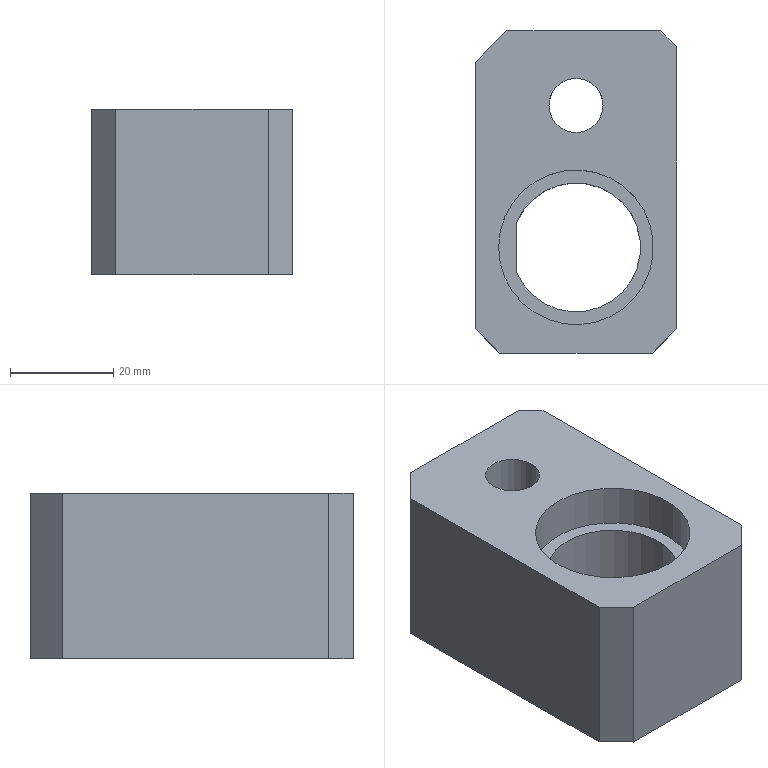Part | STEP file | lll_id3166_x_t | 1 solid | 17 faces | box 39 x 62.5 x 32 mm | volume 54047 mm3 | plane 13 | cylinder 4 | commonest cylinder face diameters 10.5 x1 17 x1 25 x1 30 x1
STEP:
#1=CARTESIAN_POINT('',(481.37,-352.399,60.5));
#2=VERTEX_POINT('',#1);
#3=CARTESIAN_POINT('',(481.37,-342.601,60.5));
#4=VERTEX_POINT('',#3);
#5=CARTESIAN_POINT('',(492.87,-347.5,60.5));
#6=DIRECTION('',(0.,0.,1.));
#7=DIRECTION('',(-1.,0.,0.));
#8=AXIS2_PLACEMENT_3D('',#5,#6,#7);
#9=CIRCLE('',#8,12.5);
#10=EDGE_CURVE('',#2,#4,#9,.T.);
#11=ORIENTED_EDGE('',*,*,#10,.T.);
#12=CARTESIAN_POINT('',(481.37,-316.275,60.5));
#13=DIRECTION('',(0.,-1.,0.));
#14=VECTOR('',#13,1.);
#15=LINE('',#12,#14);
#16=EDGE_CURVE('',#4,#2,#15,.T.);
#17=ORIENTED_EDGE('',*,*,#16,.T.);
#18=EDGE_LOOP('',(#11,#17));
#19=FACE_BOUND('',#18,.T.);
#20=CARTESIAN_POINT('',(507.613,-368.,60.5));
#21=VERTEX_POINT('',#20);
#22=CARTESIAN_POINT('',(478.128,-368.,60.5));
#23=VERTEX_POINT('',#22);
#24=CARTESIAN_POINT('',(492.87,-368.,60.5));
#25=DIRECTION('',(-1.,0.,0.));
#26=VECTOR('',#25,1.);
#27=LINE('',#24,#26);
#28=EDGE_CURVE('',#21,#23,#27,.T.);
#29=ORIENTED_EDGE('',*,*,#28,.T.);
#30=CARTESIAN_POINT('',(473.37,-363.243,60.5));
#31=VERTEX_POINT('',#30);
#32=CARTESIAN_POINT('',(425.566,-315.439,60.5));
#33=DIRECTION('',(0.7071,-0.7071,0.));
#34=VECTOR('',#33,1.);
#35=LINE('',#32,#34);
#36=EDGE_CURVE('',#31,#23,#35,.T.);
#37=ORIENTED_EDGE('',*,*,#36,.F.);
#38=CARTESIAN_POINT('',(473.37,-311.601,60.5));
#39=VERTEX_POINT('',#38);
#40=CARTESIAN_POINT('',(473.37,-347.5,60.5));
#41=DIRECTION('',(0.,1.,0.));
#42=VECTOR('',#41,1.);
#43=LINE('',#40,#42);
#44=EDGE_CURVE('',#31,#39,#43,.T.);
#45=ORIENTED_EDGE('',*,*,#44,.T.);
#46=CARTESIAN_POINT('',(479.471,-305.5,60.5));
#47=VERTEX_POINT('',#46);
#48=CARTESIAN_POINT('',(449.213,-335.758,60.5));
#49=DIRECTION('',(-0.7071,-0.7071,0.));
#50=VECTOR('',#49,1.);
#51=LINE('',#48,#50);
#52=EDGE_CURVE('',#47,#39,#51,.T.);
#53=ORIENTED_EDGE('',*,*,#52,.F.);
#54=CARTESIAN_POINT('',(509.27,-305.5,60.5));
#55=VERTEX_POINT('',#54);
#56=CARTESIAN_POINT('',(492.87,-305.5,60.5));
#57=DIRECTION('',(1.,0.,0.));
#58=VECTOR('',#57,1.);
#59=LINE('',#56,#58);
#60=EDGE_CURVE('',#47,#55,#59,.T.);
#61=ORIENTED_EDGE('',*,*,#60,.T.);
#62=CARTESIAN_POINT('',(512.37,-308.601,60.5));
#63=VERTEX_POINT('',#62);
#64=CARTESIAN_POINT('',(469.887,-266.118,60.5));
#65=DIRECTION('',(-0.7071,0.7071,0.));
#66=VECTOR('',#65,1.);
#67=LINE('',#64,#66);
#68=EDGE_CURVE('',#63,#55,#67,.T.);
#69=ORIENTED_EDGE('',*,*,#68,.F.);
#70=CARTESIAN_POINT('',(512.37,-363.243,60.5));
#71=VERTEX_POINT('',#70);
#72=CARTESIAN_POINT('',(512.37,-347.5,60.5));
#73=DIRECTION('',(0.,-1.,0.));
#74=VECTOR('',#73,1.);
#75=LINE('',#72,#74);
#76=EDGE_CURVE('',#63,#71,#75,.T.);
#77=ORIENTED_EDGE('',*,*,#76,.T.);
#78=CARTESIAN_POINT('',(492.034,-383.579,60.5));
#79=DIRECTION('',(0.7071,0.7071,0.));
#80=VECTOR('',#79,1.);
#81=LINE('',#78,#80);
#82=EDGE_CURVE('',#21,#71,#81,.T.);
#83=ORIENTED_EDGE('',*,*,#82,.F.);
#84=EDGE_LOOP('',(#29,#37,#45,#53,#61,#69,#77,#83));
#85=FACE_BOUND('',#84,.T.);
#86=CARTESIAN_POINT('',(501.37,-320.,60.5));
#87=VERTEX_POINT('',#86);
#88=CARTESIAN_POINT('',(492.87,-320.,60.5));
#89=DIRECTION('',(0.,0.,-1.));
#90=DIRECTION('',(1.,0.,0.));
#91=AXIS2_PLACEMENT_3D('',#88,#89,#90);
#92=CIRCLE('',#91,8.5);
#93=EDGE_CURVE('',#87,#87,#92,.T.);
#94=ORIENTED_EDGE('',*,*,#93,.F.);
#95=EDGE_LOOP('',(#94));
#96=FACE_BOUND('',#95,.T.);
#97=CARTESIAN_POINT('',(424.73,-316.275,60.5));
#98=DIRECTION('',(0.,0.,1.));
#99=DIRECTION('',(-1.,0.,0.));
#100=AXIS2_PLACEMENT_3D('',#97,#98,#99);
#101=PLANE('',#100);
#102=ADVANCED_FACE('',(#19,#85,#96),#101,.F.);
#103=CARTESIAN_POINT('',(477.87,-347.5,92.5));
#104=VERTEX_POINT('',#103);
#105=CARTESIAN_POINT('',(492.87,-347.5,92.5));
#106=DIRECTION('',(0.,0.,1.));
#107=DIRECTION('',(-1.,0.,0.));
#108=AXIS2_PLACEMENT_3D('',#105,#106,#107);
#109=CIRCLE('',#108,15.);
#110=EDGE_CURVE('',#104,#104,#109,.T.);
#111=ORIENTED_EDGE('',*,*,#110,.F.);
#112=EDGE_LOOP('',(#111));
#113=FACE_BOUND('',#112,.T.);
#114=CARTESIAN_POINT('',(498.12,-320.,92.5));
#115=VERTEX_POINT('',#114);
#116=CARTESIAN_POINT('',(492.87,-320.,92.5));
#117=DIRECTION('',(0.,0.,-1.));
#118=DIRECTION('',(1.,0.,0.));
#119=AXIS2_PLACEMENT_3D('',#116,#117,#118);
#120=CIRCLE('',#119,5.25);
#121=EDGE_CURVE('',#115,#115,#120,.T.);
#122=ORIENTED_EDGE('',*,*,#121,.T.);
#123=EDGE_LOOP('',(#122));
#124=FACE_BOUND('',#123,.T.);
#125=CARTESIAN_POINT('',(512.37,-363.243,92.5));
#126=VERTEX_POINT('',#125);
#127=CARTESIAN_POINT('',(512.37,-308.601,92.5));
#128=VERTEX_POINT('',#127);
#129=CARTESIAN_POINT('',(512.37,-347.5,92.5));
#130=DIRECTION('',(0.,1.,0.));
#131=VECTOR('',#130,1.);
#132=LINE('',#129,#131);
#133=EDGE_CURVE('',#126,#128,#132,.T.);
#134=ORIENTED_EDGE('',*,*,#133,.T.);
#135=CARTESIAN_POINT('',(509.27,-305.5,92.5));
#136=VERTEX_POINT('',#135);
#137=CARTESIAN_POINT('',(469.887,-266.118,92.5));
#138=DIRECTION('',(0.7071,-0.7071,0.));
#139=VECTOR('',#138,1.);
#140=LINE('',#137,#139);
#141=EDGE_CURVE('',#136,#128,#140,.T.);
#142=ORIENTED_EDGE('',*,*,#141,.F.);
#143=CARTESIAN_POINT('',(479.471,-305.5,92.5));
#144=VERTEX_POINT('',#143);
#145=CARTESIAN_POINT('',(492.87,-305.5,92.5));
#146=DIRECTION('',(-1.,0.,0.));
#147=VECTOR('',#146,1.);
#148=LINE('',#145,#147);
#149=EDGE_CURVE('',#136,#144,#148,.T.);
#150=ORIENTED_EDGE('',*,*,#149,.T.);
#151=CARTESIAN_POINT('',(473.37,-311.601,92.5));
#152=VERTEX_POINT('',#151);
#153=CARTESIAN_POINT('',(449.213,-335.758,92.5));
#154=DIRECTION('',(0.7071,0.7071,0.));
#155=VECTOR('',#154,1.);
#156=LINE('',#153,#155);
#157=EDGE_CURVE('',#152,#144,#156,.T.);
#158=ORIENTED_EDGE('',*,*,#157,.F.);
#159=CARTESIAN_POINT('',(473.37,-363.243,92.5));
#160=VERTEX_POINT('',#159);
#161=CARTESIAN_POINT('',(473.37,-347.5,92.5));
#162=DIRECTION('',(0.,-1.,0.));
#163=VECTOR('',#162,1.);
#164=LINE('',#161,#163);
#165=EDGE_CURVE('',#152,#160,#164,.T.);
#166=ORIENTED_EDGE('',*,*,#165,.T.);
#167=CARTESIAN_POINT('',(478.128,-368.,92.5));
#168=VERTEX_POINT('',#167);
#169=CARTESIAN_POINT('',(425.566,-315.439,92.5));
#170=DIRECTION('',(-0.7071,0.7071,0.));
#171=VECTOR('',#170,1.);
#172=LINE('',#169,#171);
#173=EDGE_CURVE('',#168,#160,#172,.T.);
#174=ORIENTED_EDGE('',*,*,#173,.F.);
#175=CARTESIAN_POINT('',(507.613,-368.,92.5));
#176=VERTEX_POINT('',#175);
#177=CARTESIAN_POINT('',(492.87,-368.,92.5));
#178=DIRECTION('',(1.,0.,0.));
#179=VECTOR('',#178,1.);
#180=LINE('',#177,#179);
#181=EDGE_CURVE('',#168,#176,#180,.T.);
#182=ORIENTED_EDGE('',*,*,#181,.T.);
#183=CARTESIAN_POINT('',(492.034,-383.579,92.5));
#184=DIRECTION('',(-0.7071,-0.7071,0.));
#185=VECTOR('',#184,1.);
#186=LINE('',#183,#185);
#187=EDGE_CURVE('',#126,#176,#186,.T.);
#188=ORIENTED_EDGE('',*,*,#187,.F.);
#189=EDGE_LOOP('',(#134,#142,#150,#158,#166,#174,#182,#188));
#190=FACE_BOUND('',#189,.T.);
#191=CARTESIAN_POINT('',(424.73,-316.275,92.5));
#192=DIRECTION('',(0.,0.,1.));
#193=DIRECTION('',(-1.,0.,0.));
#194=AXIS2_PLACEMENT_3D('',#191,#192,#193);
#195=PLANE('',#194);
#196=ADVANCED_FACE('',(#113,#124,#190),#195,.T.);
#197=ORIENTED_EDGE('',*,*,#181,.F.);
#198=CARTESIAN_POINT('',(478.128,-368.,-8.5));
#199=DIRECTION('',(0.,0.,1.));
#200=VECTOR('',#199,1.);
#201=LINE('',#198,#200);
#202=EDGE_CURVE('',#23,#168,#201,.T.);
#203=ORIENTED_EDGE('',*,*,#202,.F.);
#204=ORIENTED_EDGE('',*,*,#28,.F.);
#205=CARTESIAN_POINT('',(507.613,-368.,-8.5));
#206=DIRECTION('',(0.,0.,-1.));
#207=VECTOR('',#206,1.);
#208=LINE('',#205,#207);
#209=EDGE_CURVE('',#176,#21,#208,.T.);
#210=ORIENTED_EDGE('',*,*,#209,.F.);
#211=EDGE_LOOP('',(#197,#203,#204,#210));
#212=FACE_OUTER_BOUND('',#211,.T.);
#213=CARTESIAN_POINT('',(492.87,-368.,-8.5));
#214=DIRECTION('',(0.,-1.,0.));
#215=DIRECTION('',(0.,0.,-1.));
#216=AXIS2_PLACEMENT_3D('',#213,#214,#215);
#217=PLANE('',#216);
#218=ADVANCED_FACE('',(#212),#217,.T.);
#219=ORIENTED_EDGE('',*,*,#76,.F.);
#220=CARTESIAN_POINT('',(512.37,-308.601,-8.5));
#221=DIRECTION('',(0.,0.,-1.));
#222=VECTOR('',#221,1.);
#223=LINE('',#220,#222);
#224=EDGE_CURVE('',#128,#63,#223,.T.);
#225=ORIENTED_EDGE('',*,*,#224,.F.);
#226=ORIENTED_EDGE('',*,*,#133,.F.);
#227=CARTESIAN_POINT('',(512.37,-363.243,-8.5));
#228=DIRECTION('',(0.,0.,1.));
#229=VECTOR('',#228,1.);
#230=LINE('',#227,#229);
#231=EDGE_CURVE('',#71,#126,#230,.T.);
#232=ORIENTED_EDGE('',*,*,#231,.F.);
#233=EDGE_LOOP('',(#219,#225,#226,#232));
#234=FACE_OUTER_BOUND('',#233,.T.);
#235=CARTESIAN_POINT('',(512.37,-347.5,-8.5));
#236=DIRECTION('',(1.,0.,0.));
#237=DIRECTION('',(0.,0.,1.));
#238=AXIS2_PLACEMENT_3D('',#235,#236,#237);
#239=PLANE('',#238);
#240=ADVANCED_FACE('',(#234),#239,.T.);
#241=ORIENTED_EDGE('',*,*,#149,.F.);
#242=CARTESIAN_POINT('',(509.27,-305.5,-8.5));
#243=DIRECTION('',(0.,0.,1.));
#244=VECTOR('',#243,1.);
#245=LINE('',#242,#244);
#246=EDGE_CURVE('',#55,#136,#245,.T.);
#247=ORIENTED_EDGE('',*,*,#246,.F.);
#248=ORIENTED_EDGE('',*,*,#60,.F.);
#249=CARTESIAN_POINT('',(479.471,-305.5,-8.5));
#250=DIRECTION('',(0.,0.,-1.));
#251=VECTOR('',#250,1.);
#252=LINE('',#249,#251);
#253=EDGE_CURVE('',#144,#47,#252,.T.);
#254=ORIENTED_EDGE('',*,*,#253,.F.);
#255=EDGE_LOOP('',(#241,#247,#248,#254));
#256=FACE_OUTER_BOUND('',#255,.T.);
#257=CARTESIAN_POINT('',(492.87,-305.5,-8.5));
#258=DIRECTION('',(0.,1.,0.));
#259=DIRECTION('',(0.,0.,1.));
#260=AXIS2_PLACEMENT_3D('',#257,#258,#259);
#261=PLANE('',#260);
#262=ADVANCED_FACE('',(#256),#261,.T.);
#263=ORIENTED_EDGE('',*,*,#165,.F.);
#264=CARTESIAN_POINT('',(473.37,-311.601,-8.5));
#265=DIRECTION('',(0.,0.,1.));
#266=VECTOR('',#265,1.);
#267=LINE('',#264,#266);
#268=EDGE_CURVE('',#39,#152,#267,.T.);
#269=ORIENTED_EDGE('',*,*,#268,.F.);
#270=ORIENTED_EDGE('',*,*,#44,.F.);
#271=CARTESIAN_POINT('',(473.37,-363.243,-8.5));
#272=DIRECTION('',(0.,0.,-1.));
#273=VECTOR('',#272,1.);
#274=LINE('',#271,#273);
#275=EDGE_CURVE('',#160,#31,#274,.T.);
#276=ORIENTED_EDGE('',*,*,#275,.F.);
#277=EDGE_LOOP('',(#263,#269,#270,#276));
#278=FACE_OUTER_BOUND('',#277,.T.);
#279=CARTESIAN_POINT('',(473.37,-347.5,-8.5));
#280=DIRECTION('',(-1.,0.,0.));
#281=DIRECTION('',(0.,0.,-1.));
#282=AXIS2_PLACEMENT_3D('',#279,#280,#281);
#283=PLANE('',#282);
#284=ADVANCED_FACE('',(#278),#283,.T.);
#285=ORIENTED_EDGE('',*,*,#121,.F.);
#286=EDGE_LOOP('',(#285));
#287=FACE_BOUND('',#286,.T.);
#288=CARTESIAN_POINT('',(498.12,-320.,77.5));
#289=VERTEX_POINT('',#288);
#290=CARTESIAN_POINT('',(492.87,-320.,77.5));
#291=DIRECTION('',(0.,0.,1.));
#292=DIRECTION('',(1.,0.,0.));
#293=AXIS2_PLACEMENT_3D('',#290,#291,#292);
#294=CIRCLE('',#293,5.25);
#295=EDGE_CURVE('',#289,#289,#294,.T.);
#296=ORIENTED_EDGE('',*,*,#295,.F.);
#297=EDGE_LOOP('',(#296));
#298=FACE_BOUND('',#297,.T.);
#299=CARTESIAN_POINT('',(492.87,-320.,160.5));
#300=DIRECTION('',(0.,0.,1.));
#301=DIRECTION('',(-1.,0.,0.));
#302=AXIS2_PLACEMENT_3D('',#299,#300,#301);
#303=CYLINDRICAL_SURFACE('',#302,5.25);
#304=ADVANCED_FACE('',(#287,#298),#303,.F.);
#305=ORIENTED_EDGE('',*,*,#295,.T.);
#306=EDGE_LOOP('',(#305));
#307=FACE_BOUND('',#306,.T.);
#308=CARTESIAN_POINT('',(501.37,-320.,77.5));
#309=VERTEX_POINT('',#308);
#310=CARTESIAN_POINT('',(492.87,-320.,77.5));
#311=DIRECTION('',(0.,0.,1.));
#312=DIRECTION('',(1.,0.,0.));
#313=AXIS2_PLACEMENT_3D('',#310,#311,#312);
#314=CIRCLE('',#313,8.5);
#315=EDGE_CURVE('',#309,#309,#314,.T.);
#316=ORIENTED_EDGE('',*,*,#315,.F.);
#317=EDGE_LOOP('',(#316));
#318=FACE_BOUND('',#317,.T.);
#319=CARTESIAN_POINT('',(492.87,-320.,77.5));
#320=DIRECTION('',(0.,0.,1.));
#321=DIRECTION('',(-1.,0.,0.));
#322=AXIS2_PLACEMENT_3D('',#319,#320,#321);
#323=PLANE('',#322);
#324=ADVANCED_FACE('',(#307,#318),#323,.F.);
#325=ORIENTED_EDGE('',*,*,#315,.T.);
#326=EDGE_LOOP('',(#325));
#327=FACE_BOUND('',#326,.T.);
#328=ORIENTED_EDGE('',*,*,#93,.T.);
#329=EDGE_LOOP('',(#328));
#330=FACE_BOUND('',#329,.T.);
#331=CARTESIAN_POINT('',(492.87,-320.,60.5));
#332=DIRECTION('',(0.,0.,1.));
#333=DIRECTION('',(-1.,0.,0.));
#334=AXIS2_PLACEMENT_3D('',#331,#332,#333);
#335=CYLINDRICAL_SURFACE('',#334,8.5);
#336=ADVANCED_FACE('',(#327,#330),#335,.F.);
#337=ORIENTED_EDGE('',*,*,#68,.T.);
#338=ORIENTED_EDGE('',*,*,#246,.T.);
#339=ORIENTED_EDGE('',*,*,#141,.T.);
#340=ORIENTED_EDGE('',*,*,#224,.T.);
#341=EDGE_LOOP('',(#337,#338,#339,#340));
#342=FACE_OUTER_BOUND('',#341,.T.);
#343=CARTESIAN_POINT('',(507.32,-303.55,-8.5));
#344=DIRECTION('',(-0.7071,-0.7071,0.));
#345=DIRECTION('',(0.,0.,1.));
#346=AXIS2_PLACEMENT_3D('',#343,#344,#345);
#347=PLANE('',#346);
#348=ADVANCED_FACE('',(#342),#347,.F.);
#349=ORIENTED_EDGE('',*,*,#157,.T.);
#350=ORIENTED_EDGE('',*,*,#253,.T.);
#351=ORIENTED_EDGE('',*,*,#52,.T.);
#352=ORIENTED_EDGE('',*,*,#268,.T.);
#353=EDGE_LOOP('',(#349,#350,#351,#352));
#354=FACE_OUTER_BOUND('',#353,.T.);
#355=CARTESIAN_POINT('',(481.421,-303.55,-8.5));
#356=DIRECTION('',(0.7071,-0.7071,0.));
#357=DIRECTION('',(0.,0.,-1.));
#358=AXIS2_PLACEMENT_3D('',#355,#356,#357);
#359=PLANE('',#358);
#360=ADVANCED_FACE('',(#354),#359,.F.);
#361=CARTESIAN_POINT('',(481.37,-352.399,84.3));
#362=VERTEX_POINT('',#361);
#363=CARTESIAN_POINT('',(481.37,-342.601,84.3));
#364=VERTEX_POINT('',#363);
#365=CARTESIAN_POINT('',(481.37,-347.5,84.3));
#366=DIRECTION('',(0.,1.,0.));
#367=VECTOR('',#366,1.);
#368=LINE('',#365,#367);
#369=EDGE_CURVE('',#362,#364,#368,.T.);
#370=ORIENTED_EDGE('',*,*,#369,.T.);
#371=CARTESIAN_POINT('',(492.87,-347.5,84.3));
#372=DIRECTION('',(0.,0.,1.));
#373=DIRECTION('',(1.,0.,0.));
#374=AXIS2_PLACEMENT_3D('',#371,#372,#373);
#375=CIRCLE('',#374,12.5);
#376=EDGE_CURVE('',#362,#364,#375,.T.);
#377=ORIENTED_EDGE('',*,*,#376,.F.);
#378=EDGE_LOOP('',(#370,#377));
#379=FACE_BOUND('',#378,.T.);
#380=CARTESIAN_POINT('',(477.87,-347.5,84.3));
#381=VERTEX_POINT('',#380);
#382=CARTESIAN_POINT('',(492.87,-347.5,84.3));
#383=DIRECTION('',(0.,0.,-1.));
#384=DIRECTION('',(1.,0.,0.));
#385=AXIS2_PLACEMENT_3D('',#382,#383,#384);
#386=CIRCLE('',#385,15.);
#387=EDGE_CURVE('',#381,#381,#386,.T.);
#388=ORIENTED_EDGE('',*,*,#387,.F.);
#389=EDGE_LOOP('',(#388));
#390=FACE_BOUND('',#389,.T.);
#391=CARTESIAN_POINT('',(492.87,-347.5,84.3));
#392=DIRECTION('',(0.,0.,1.));
#393=DIRECTION('',(-1.,0.,0.));
#394=AXIS2_PLACEMENT_3D('',#391,#392,#393);
#395=PLANE('',#394);
#396=ADVANCED_FACE('',(#379,#390),#395,.T.);
#397=ORIENTED_EDGE('',*,*,#376,.T.);
#398=CARTESIAN_POINT('',(481.37,-342.601,-7.5));
#399=DIRECTION('',(0.,0.,-1.));
#400=VECTOR('',#399,1.);
#401=LINE('',#398,#400);
#402=EDGE_CURVE('',#364,#4,#401,.T.);
#403=ORIENTED_EDGE('',*,*,#402,.T.);
#404=ORIENTED_EDGE('',*,*,#10,.F.);
#405=CARTESIAN_POINT('',(481.37,-352.399,-7.5));
#406=DIRECTION('',(0.,0.,1.));
#407=VECTOR('',#406,1.);
#408=LINE('',#405,#407);
#409=EDGE_CURVE('',#2,#362,#408,.T.);
#410=ORIENTED_EDGE('',*,*,#409,.T.);
#411=EDGE_LOOP('',(#397,#403,#404,#410));
#412=FACE_OUTER_BOUND('',#411,.T.);
#413=CARTESIAN_POINT('',(492.87,-347.5,124.8));
#414=DIRECTION('',(0.,0.,-1.));
#415=DIRECTION('',(1.,0.,0.));
#416=AXIS2_PLACEMENT_3D('',#413,#414,#415);
#417=CYLINDRICAL_SURFACE('',#416,12.5);
#418=ADVANCED_FACE('',(#412),#417,.F.);
#419=ORIENTED_EDGE('',*,*,#82,.T.);
#420=ORIENTED_EDGE('',*,*,#231,.T.);
#421=ORIENTED_EDGE('',*,*,#187,.T.);
#422=ORIENTED_EDGE('',*,*,#209,.T.);
#423=EDGE_LOOP('',(#419,#420,#421,#422));
#424=FACE_OUTER_BOUND('',#423,.T.);
#425=CARTESIAN_POINT('',(511.492,-364.121,-8.5));
#426=DIRECTION('',(-0.7071,0.7071,0.));
#427=DIRECTION('',(0.,0.,1.));
#428=AXIS2_PLACEMENT_3D('',#425,#426,#427);
#429=PLANE('',#428);
#430=ADVANCED_FACE('',(#424),#429,.F.);
#431=ORIENTED_EDGE('',*,*,#36,.T.);
#432=ORIENTED_EDGE('',*,*,#202,.T.);
#433=ORIENTED_EDGE('',*,*,#173,.T.);
#434=ORIENTED_EDGE('',*,*,#275,.T.);
#435=EDGE_LOOP('',(#431,#432,#433,#434));
#436=FACE_OUTER_BOUND('',#435,.T.);
#437=CARTESIAN_POINT('',(477.249,-367.121,-8.5));
#438=DIRECTION('',(0.7071,0.7071,0.));
#439=DIRECTION('',(0.,0.,1.));
#440=AXIS2_PLACEMENT_3D('',#437,#438,#439);
#441=PLANE('',#440);
#442=ADVANCED_FACE('',(#436),#441,.F.);
#443=ORIENTED_EDGE('',*,*,#387,.T.);
#444=EDGE_LOOP('',(#443));
#445=FACE_BOUND('',#444,.T.);
#446=ORIENTED_EDGE('',*,*,#110,.T.);
#447=EDGE_LOOP('',(#446));
#448=FACE_BOUND('',#447,.T.);
#449=CARTESIAN_POINT('',(492.87,-347.5,-7.5));
#450=DIRECTION('',(0.,0.,1.));
#451=DIRECTION('',(-1.,0.,0.));
#452=AXIS2_PLACEMENT_3D('',#449,#450,#451);
#453=CYLINDRICAL_SURFACE('',#452,15.);
#454=ADVANCED_FACE('',(#445,#448),#453,.F.);
#455=ORIENTED_EDGE('',*,*,#16,.F.);
#456=ORIENTED_EDGE('',*,*,#402,.F.);
#457=ORIENTED_EDGE('',*,*,#369,.F.);
#458=ORIENTED_EDGE('',*,*,#409,.F.);
#459=EDGE_LOOP('',(#455,#456,#457,#458));
#460=FACE_OUTER_BOUND('',#459,.T.);
#461=CARTESIAN_POINT('',(481.37,-347.5,92.5));
#462=DIRECTION('',(-1.,0.,0.));
#463=DIRECTION('',(0.,0.,-1.));
#464=AXIS2_PLACEMENT_3D('',#461,#462,#463);
#465=PLANE('',#464);
#466=ADVANCED_FACE('',(#460),#465,.F.);
#467=CLOSED_SHELL('',(#102,#196,#218,#240,#262,#284,#304,#324,#336,#348,#360,#396,#418,#430,#442,#454,#466));
#468=MANIFOLD_SOLID_BREP('',#467);
#469=(LENGTH_UNIT()NAMED_UNIT(*)SI_UNIT(.MILLI.,.METRE.));
#470=UNCERTAINTY_MEASURE_WITH_UNIT(LENGTH_MEASURE(0.00002),#469,'','');
#471=(NAMED_UNIT(*)PLANE_ANGLE_UNIT()SI_UNIT($,.RADIAN.));
#472=PLANE_ANGLE_MEASURE_WITH_UNIT(PLANE_ANGLE_MEASURE(0.01745),#471);
#473=DIMENSIONAL_EXPONENTS(0.,0.,0.,0.,0.,0.,0.);
#474=(CONVERSION_BASED_UNIT('DEGREE',#472)NAMED_UNIT(#473)PLANE_ANGLE_UNIT());
#475=(NAMED_UNIT(*)SI_UNIT($,.STERADIAN.)SOLID_ANGLE_UNIT());
#476=(GEOMETRIC_REPRESENTATION_CONTEXT(3)GLOBAL_UNCERTAINTY_ASSIGNED_CONTEXT((#470))GLOBAL_UNIT_ASSIGNED_CONTEXT((#469,#474,#475))REPRESENTATION_CONTEXT('',''));
#477=ADVANCED_BREP_SHAPE_REPRESENTATION('',(#468),#476);